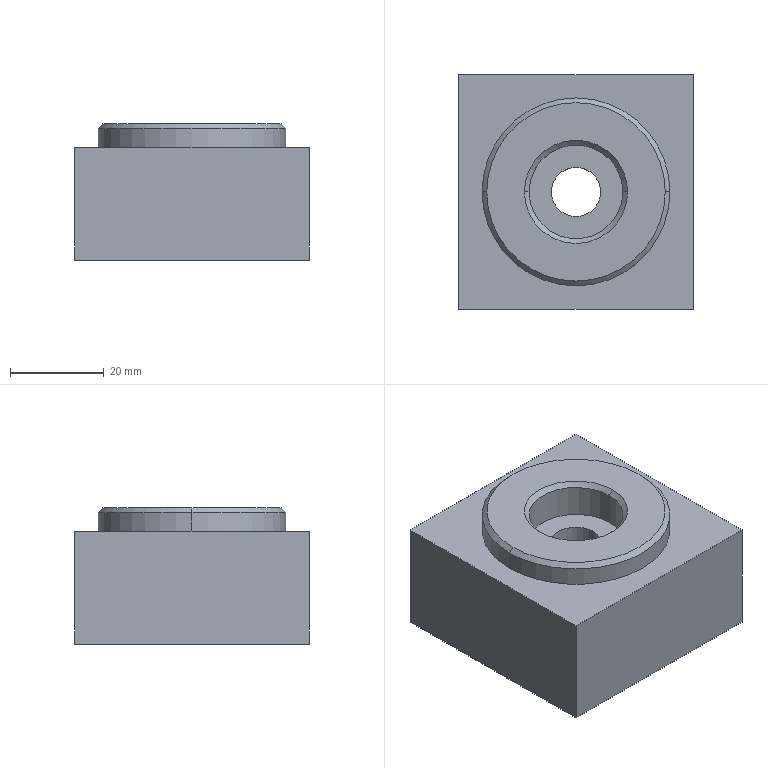Part | SolidWorks | features ICE 3, Chamfer 2, Extrusion 1 | 1 solid | 18 faces | box 50 x 50 x 29 mm | volume 61857 mm3 | plane 8 | cylinder 6 | cone 4 | commonest cylinder face diameters 10.5 x2 20 x2 40 x2
STEP:
#1=CARTESIAN_POINT('',(19.,0.,29.));
#2=VERTEX_POINT('',#1);
#3=CARTESIAN_POINT('',(-19.,0.,29.));
#4=VERTEX_POINT('',#3);
#5=CARTESIAN_POINT('',(0.,0.,29.));
#6=DIRECTION('',(0.,0.,1.));
#7=DIRECTION('',(1.,0.,0.));
#8=AXIS2_PLACEMENT_3D('',#5,#6,#7);
#9=CIRCLE('',#8,19.);
#10=EDGE_CURVE('',#2,#4,#9,.T.);
#11=ORIENTED_EDGE('',*,*,#10,.F.);
#12=CARTESIAN_POINT('',(20.,0.,28.));
#13=VERTEX_POINT('',#12);
#14=CARTESIAN_POINT('',(19.,0.,29.));
#15=DIRECTION('',(0.7071,0.,-0.7071));
#16=VECTOR('',#15,1000.);
#17=LINE('',#14,#16);
#18=EDGE_CURVE('',#2,#13,#17,.T.);
#19=ORIENTED_EDGE('',*,*,#18,.T.);
#20=CARTESIAN_POINT('',(-20.,0.,28.));
#21=VERTEX_POINT('',#20);
#22=CARTESIAN_POINT('',(0.,0.,28.));
#23=DIRECTION('',(0.,0.,-1.));
#24=DIRECTION('',(1.,0.,0.));
#25=AXIS2_PLACEMENT_3D('',#22,#23,#24);
#26=CIRCLE('',#25,20.);
#27=EDGE_CURVE('',#21,#13,#26,.T.);
#28=ORIENTED_EDGE('',*,*,#27,.F.);
#29=CARTESIAN_POINT('',(-19.,0.,29.));
#30=DIRECTION('',(-0.7071,0.,-0.7071));
#31=VECTOR('',#30,1000.);
#32=LINE('',#29,#31);
#33=EDGE_CURVE('',#4,#21,#32,.T.);
#34=ORIENTED_EDGE('',*,*,#33,.F.);
#35=EDGE_LOOP('',(#11,#19,#28,#34));
#36=FACE_OUTER_BOUND('',#35,.T.);
#37=CARTESIAN_POINT('',(0.,0.,29.));
#38=DIRECTION('',(0.,0.,-1.));
#39=DIRECTION('',(-1.,0.,0.));
#40=AXIS2_PLACEMENT_3D('',#37,#38,#39);
#41=CONICAL_SURFACE('',#40,19.,0.7854);
#42=ADVANCED_FACE('',(#36),#41,.T.);
#43=CARTESIAN_POINT('',(20.,0.,24.));
#44=VERTEX_POINT('',#43);
#45=CARTESIAN_POINT('',(-20.,0.,24.));
#46=VERTEX_POINT('',#45);
#47=CARTESIAN_POINT('',(0.,0.,24.));
#48=DIRECTION('',(0.,0.,1.));
#49=DIRECTION('',(1.,0.,0.));
#50=AXIS2_PLACEMENT_3D('',#47,#48,#49);
#51=CIRCLE('',#50,20.);
#52=EDGE_CURVE('',#44,#46,#51,.T.);
#53=ORIENTED_EDGE('',*,*,#52,.T.);
#54=CARTESIAN_POINT('',(-20.,0.,24.));
#55=DIRECTION('',(0.,0.,1.));
#56=VECTOR('',#55,1000.);
#57=LINE('',#54,#56);
#58=EDGE_CURVE('',#46,#21,#57,.T.);
#59=ORIENTED_EDGE('',*,*,#58,.T.);
#60=ORIENTED_EDGE('',*,*,#27,.T.);
#61=CARTESIAN_POINT('',(20.,0.,24.));
#62=DIRECTION('',(0.,0.,1.));
#63=VECTOR('',#62,1000.);
#64=LINE('',#61,#63);
#65=EDGE_CURVE('',#44,#13,#64,.T.);
#66=ORIENTED_EDGE('',*,*,#65,.F.);
#67=EDGE_LOOP('',(#53,#59,#60,#66));
#68=FACE_OUTER_BOUND('',#67,.T.);
#69=CARTESIAN_POINT('',(0.,0.,24.));
#70=DIRECTION('',(0.,0.,1.));
#71=DIRECTION('',(1.,0.,0.));
#72=AXIS2_PLACEMENT_3D('',#69,#70,#71);
#73=CYLINDRICAL_SURFACE('',#72,20.);
#74=ADVANCED_FACE('',(#68),#73,.T.);
#75=CARTESIAN_POINT('',(-10.,0.,28.));
#76=VERTEX_POINT('',#75);
#77=CARTESIAN_POINT('',(10.,0.,28.));
#78=VERTEX_POINT('',#77);
#79=CARTESIAN_POINT('',(0.,0.,28.));
#80=DIRECTION('',(0.,0.,1.));
#81=DIRECTION('',(1.,0.,0.));
#82=AXIS2_PLACEMENT_3D('',#79,#80,#81);
#83=CIRCLE('',#82,10.);
#84=EDGE_CURVE('',#76,#78,#83,.T.);
#85=ORIENTED_EDGE('',*,*,#84,.F.);
#86=CARTESIAN_POINT('',(-11.,0.,29.));
#87=VERTEX_POINT('',#86);
#88=CARTESIAN_POINT('',(-10.,0.,28.));
#89=DIRECTION('',(-0.7071,0.,0.7071));
#90=VECTOR('',#89,1000.);
#91=LINE('',#88,#90);
#92=EDGE_CURVE('',#76,#87,#91,.T.);
#93=ORIENTED_EDGE('',*,*,#92,.T.);
#94=CARTESIAN_POINT('',(11.,0.,29.));
#95=VERTEX_POINT('',#94);
#96=CARTESIAN_POINT('',(0.,0.,29.));
#97=DIRECTION('',(0.,0.,-1.));
#98=DIRECTION('',(1.,0.,0.));
#99=AXIS2_PLACEMENT_3D('',#96,#97,#98);
#100=CIRCLE('',#99,11.);
#101=EDGE_CURVE('',#95,#87,#100,.T.);
#102=ORIENTED_EDGE('',*,*,#101,.F.);
#103=CARTESIAN_POINT('',(10.,0.,28.));
#104=DIRECTION('',(0.7071,0.,0.7071));
#105=VECTOR('',#104,1000.);
#106=LINE('',#103,#105);
#107=EDGE_CURVE('',#78,#95,#106,.T.);
#108=ORIENTED_EDGE('',*,*,#107,.F.);
#109=EDGE_LOOP('',(#85,#93,#102,#108));
#110=FACE_OUTER_BOUND('',#109,.T.);
#111=CARTESIAN_POINT('',(0.,0.,28.));
#112=DIRECTION('',(0.,0.,1.));
#113=DIRECTION('',(1.,0.,0.));
#114=AXIS2_PLACEMENT_3D('',#111,#112,#113);
#115=CONICAL_SURFACE('',#114,10.,0.7854);
#116=ADVANCED_FACE('',(#110),#115,.F.);
#117=CARTESIAN_POINT('',(5.25,0.,21.));
#118=VERTEX_POINT('',#117);
#119=CARTESIAN_POINT('',(-5.25,0.,21.));
#120=VERTEX_POINT('',#119);
#121=CARTESIAN_POINT('',(0.,0.,21.));
#122=DIRECTION('',(0.,0.,-1.));
#123=DIRECTION('',(-1.,0.,0.));
#124=AXIS2_PLACEMENT_3D('',#121,#122,#123);
#125=CIRCLE('',#124,5.25);
#126=EDGE_CURVE('',#118,#120,#125,.T.);
#127=ORIENTED_EDGE('',*,*,#126,.F.);
#128=CARTESIAN_POINT('',(5.25,0.,0.));
#129=VERTEX_POINT('',#128);
#130=CARTESIAN_POINT('',(5.25,0.,21.));
#131=DIRECTION('',(0.,0.,-1.));
#132=VECTOR('',#131,1000.);
#133=LINE('',#130,#132);
#134=EDGE_CURVE('',#118,#129,#133,.T.);
#135=ORIENTED_EDGE('',*,*,#134,.T.);
#136=CARTESIAN_POINT('',(-5.25,0.,0.));
#137=VERTEX_POINT('',#136);
#138=CARTESIAN_POINT('',(0.,0.,0.));
#139=DIRECTION('',(0.,0.,-1.));
#140=DIRECTION('',(-1.,0.,0.));
#141=AXIS2_PLACEMENT_3D('',#138,#139,#140);
#142=CIRCLE('',#141,5.25);
#143=EDGE_CURVE('',#129,#137,#142,.T.);
#144=ORIENTED_EDGE('',*,*,#143,.T.);
#145=CARTESIAN_POINT('',(-5.25,0.,21.));
#146=DIRECTION('',(0.,0.,-1.));
#147=VECTOR('',#146,1000.);
#148=LINE('',#145,#147);
#149=EDGE_CURVE('',#120,#137,#148,.T.);
#150=ORIENTED_EDGE('',*,*,#149,.F.);
#151=EDGE_LOOP('',(#127,#135,#144,#150));
#152=FACE_OUTER_BOUND('',#151,.T.);
#153=CARTESIAN_POINT('',(0.,0.,21.));
#154=DIRECTION('',(0.,0.,-1.));
#155=DIRECTION('',(-1.,0.,0.));
#156=AXIS2_PLACEMENT_3D('',#153,#154,#155);
#157=CYLINDRICAL_SURFACE('',#156,5.25);
#158=ADVANCED_FACE('',(#152),#157,.F.);
#159=CARTESIAN_POINT('',(-10.,0.,21.));
#160=VERTEX_POINT('',#159);
#161=CARTESIAN_POINT('',(10.,0.,21.));
#162=VERTEX_POINT('',#161);
#163=CARTESIAN_POINT('',(0.,0.,21.));
#164=DIRECTION('',(0.,0.,1.));
#165=DIRECTION('',(1.,0.,0.));
#166=AXIS2_PLACEMENT_3D('',#163,#164,#165);
#167=CIRCLE('',#166,10.);
#168=EDGE_CURVE('',#160,#162,#167,.T.);
#169=ORIENTED_EDGE('',*,*,#168,.F.);
#170=CARTESIAN_POINT('',(-10.,0.,21.));
#171=DIRECTION('',(0.,0.,1.));
#172=VECTOR('',#171,1000.);
#173=LINE('',#170,#172);
#174=EDGE_CURVE('',#160,#76,#173,.T.);
#175=ORIENTED_EDGE('',*,*,#174,.T.);
#176=ORIENTED_EDGE('',*,*,#84,.T.);
#177=CARTESIAN_POINT('',(10.,0.,21.));
#178=DIRECTION('',(0.,0.,1.));
#179=VECTOR('',#178,1000.);
#180=LINE('',#177,#179);
#181=EDGE_CURVE('',#162,#78,#180,.T.);
#182=ORIENTED_EDGE('',*,*,#181,.F.);
#183=EDGE_LOOP('',(#169,#175,#176,#182));
#184=FACE_OUTER_BOUND('',#183,.T.);
#185=CARTESIAN_POINT('',(0.,0.,21.));
#186=DIRECTION('',(0.,0.,1.));
#187=DIRECTION('',(1.,0.,0.));
#188=AXIS2_PLACEMENT_3D('',#185,#186,#187);
#189=CYLINDRICAL_SURFACE('',#188,10.);
#190=ADVANCED_FACE('',(#184),#189,.F.);
#191=CARTESIAN_POINT('',(25.,-25.,24.));
#192=VERTEX_POINT('',#191);
#193=CARTESIAN_POINT('',(25.,25.,24.));
#194=VERTEX_POINT('',#193);
#195=CARTESIAN_POINT('',(25.,25.,24.));
#196=DIRECTION('',(0.,1.,0.));
#197=VECTOR('',#196,1000.);
#198=LINE('',#195,#197);
#199=EDGE_CURVE('',#192,#194,#198,.T.);
#200=ORIENTED_EDGE('',*,*,#199,.F.);
#201=CARTESIAN_POINT('',(25.,-25.,0.));
#202=VERTEX_POINT('',#201);
#203=CARTESIAN_POINT('',(25.,-25.,29.));
#204=DIRECTION('',(0.,0.,-1.));
#205=VECTOR('',#204,1000.);
#206=LINE('',#203,#205);
#207=EDGE_CURVE('',#192,#202,#206,.T.);
#208=ORIENTED_EDGE('',*,*,#207,.T.);
#209=CARTESIAN_POINT('',(25.,25.,0.));
#210=VERTEX_POINT('',#209);
#211=CARTESIAN_POINT('',(25.,25.,0.));
#212=DIRECTION('',(0.,1.,0.));
#213=VECTOR('',#212,1000.);
#214=LINE('',#211,#213);
#215=EDGE_CURVE('',#202,#210,#214,.T.);
#216=ORIENTED_EDGE('',*,*,#215,.T.);
#217=CARTESIAN_POINT('',(25.,25.,29.));
#218=DIRECTION('',(0.,0.,-1.));
#219=VECTOR('',#218,1000.);
#220=LINE('',#217,#219);
#221=EDGE_CURVE('',#194,#210,#220,.T.);
#222=ORIENTED_EDGE('',*,*,#221,.F.);
#223=EDGE_LOOP('',(#200,#208,#216,#222));
#224=FACE_OUTER_BOUND('',#223,.T.);
#225=CARTESIAN_POINT('',(25.,25.,29.));
#226=DIRECTION('',(-1.,0.,0.));
#227=DIRECTION('',(0.,-1.,0.));
#228=AXIS2_PLACEMENT_3D('',#225,#226,#227);
#229=PLANE('',#228);
#230=ADVANCED_FACE('',(#224),#229,.F.);
#231=CARTESIAN_POINT('',(-25.,25.,24.));
#232=VERTEX_POINT('',#231);
#233=CARTESIAN_POINT('',(-25.,25.,24.));
#234=DIRECTION('',(-1.,0.,0.));
#235=VECTOR('',#234,1000.);
#236=LINE('',#233,#235);
#237=EDGE_CURVE('',#194,#232,#236,.T.);
#238=ORIENTED_EDGE('',*,*,#237,.F.);
#239=ORIENTED_EDGE('',*,*,#221,.T.);
#240=CARTESIAN_POINT('',(-25.,25.,0.));
#241=VERTEX_POINT('',#240);
#242=CARTESIAN_POINT('',(-25.,25.,0.));
#243=DIRECTION('',(-1.,0.,0.));
#244=VECTOR('',#243,1000.);
#245=LINE('',#242,#244);
#246=EDGE_CURVE('',#210,#241,#245,.T.);
#247=ORIENTED_EDGE('',*,*,#246,.T.);
#248=CARTESIAN_POINT('',(-25.,25.,29.));
#249=DIRECTION('',(0.,0.,-1.));
#250=VECTOR('',#249,1000.);
#251=LINE('',#248,#250);
#252=EDGE_CURVE('',#232,#241,#251,.T.);
#253=ORIENTED_EDGE('',*,*,#252,.F.);
#254=EDGE_LOOP('',(#238,#239,#247,#253));
#255=FACE_OUTER_BOUND('',#254,.T.);
#256=CARTESIAN_POINT('',(-25.,25.,29.));
#257=DIRECTION('',(0.,-1.,0.));
#258=DIRECTION('',(0.,0.,-1.));
#259=AXIS2_PLACEMENT_3D('',#256,#257,#258);
#260=PLANE('',#259);
#261=ADVANCED_FACE('',(#255),#260,.F.);
#262=CARTESIAN_POINT('',(-25.,-25.,24.));
#263=VERTEX_POINT('',#262);
#264=CARTESIAN_POINT('',(-25.,25.,24.));
#265=DIRECTION('',(0.,-1.,0.));
#266=VECTOR('',#265,1000.);
#267=LINE('',#264,#266);
#268=EDGE_CURVE('',#232,#263,#267,.T.);
#269=ORIENTED_EDGE('',*,*,#268,.F.);
#270=ORIENTED_EDGE('',*,*,#252,.T.);
#271=CARTESIAN_POINT('',(-25.,-25.,0.));
#272=VERTEX_POINT('',#271);
#273=CARTESIAN_POINT('',(-25.,25.,0.));
#274=DIRECTION('',(0.,-1.,0.));
#275=VECTOR('',#274,1000.);
#276=LINE('',#273,#275);
#277=EDGE_CURVE('',#241,#272,#276,.T.);
#278=ORIENTED_EDGE('',*,*,#277,.T.);
#279=CARTESIAN_POINT('',(-25.,-25.,29.));
#280=DIRECTION('',(0.,0.,-1.));
#281=VECTOR('',#280,1000.);
#282=LINE('',#279,#281);
#283=EDGE_CURVE('',#263,#272,#282,.T.);
#284=ORIENTED_EDGE('',*,*,#283,.F.);
#285=EDGE_LOOP('',(#269,#270,#278,#284));
#286=FACE_OUTER_BOUND('',#285,.T.);
#287=CARTESIAN_POINT('',(-25.,25.,29.));
#288=DIRECTION('',(1.,0.,0.));
#289=DIRECTION('',(0.,1.,0.));
#290=AXIS2_PLACEMENT_3D('',#287,#288,#289);
#291=PLANE('',#290);
#292=ADVANCED_FACE('',(#286),#291,.F.);
#293=CARTESIAN_POINT('',(-25.,-25.,24.));
#294=DIRECTION('',(1.,0.,0.));
#295=VECTOR('',#294,1000.);
#296=LINE('',#293,#295);
#297=EDGE_CURVE('',#263,#192,#296,.T.);
#298=ORIENTED_EDGE('',*,*,#297,.F.);
#299=ORIENTED_EDGE('',*,*,#283,.T.);
#300=CARTESIAN_POINT('',(-25.,-25.,0.));
#301=DIRECTION('',(1.,0.,0.));
#302=VECTOR('',#301,1000.);
#303=LINE('',#300,#302);
#304=EDGE_CURVE('',#272,#202,#303,.T.);
#305=ORIENTED_EDGE('',*,*,#304,.T.);
#306=ORIENTED_EDGE('',*,*,#207,.F.);
#307=EDGE_LOOP('',(#298,#299,#305,#306));
#308=FACE_OUTER_BOUND('',#307,.T.);
#309=CARTESIAN_POINT('',(-25.,-25.,29.));
#310=DIRECTION('',(0.,1.,0.));
#311=DIRECTION('',(0.,0.,1.));
#312=AXIS2_PLACEMENT_3D('',#309,#310,#311);
#313=PLANE('',#312);
#314=ADVANCED_FACE('',(#308),#313,.F.);
#315=CARTESIAN_POINT('',(0.,0.,29.));
#316=DIRECTION('',(0.,0.,1.));
#317=DIRECTION('',(1.,0.,0.));
#318=AXIS2_PLACEMENT_3D('',#315,#316,#317);
#319=CIRCLE('',#318,19.);
#320=EDGE_CURVE('',#4,#2,#319,.T.);
#321=ORIENTED_EDGE('',*,*,#320,.T.);
#322=ORIENTED_EDGE('',*,*,#10,.T.);
#323=EDGE_LOOP('',(#321,#322));
#324=FACE_OUTER_BOUND('',#323,.T.);
#325=ORIENTED_EDGE('',*,*,#101,.T.);
#326=CARTESIAN_POINT('',(0.,0.,29.));
#327=DIRECTION('',(0.,0.,-1.));
#328=DIRECTION('',(1.,0.,0.));
#329=AXIS2_PLACEMENT_3D('',#326,#327,#328);
#330=CIRCLE('',#329,11.);
#331=EDGE_CURVE('',#87,#95,#330,.T.);
#332=ORIENTED_EDGE('',*,*,#331,.T.);
#333=EDGE_LOOP('',(#325,#332));
#334=FACE_BOUND('',#333,.T.);
#335=CARTESIAN_POINT('',(0.,0.,29.));
#336=DIRECTION('',(0.,0.,1.));
#337=DIRECTION('',(1.,0.,0.));
#338=AXIS2_PLACEMENT_3D('',#335,#336,#337);
#339=PLANE('',#338);
#340=ADVANCED_FACE('',(#324,#334),#339,.T.);
#341=CARTESIAN_POINT('',(0.,0.,0.));
#342=DIRECTION('',(0.,0.,-1.));
#343=DIRECTION('',(-1.,0.,0.));
#344=AXIS2_PLACEMENT_3D('',#341,#342,#343);
#345=CIRCLE('',#344,5.25);
#346=EDGE_CURVE('',#137,#129,#345,.T.);
#347=ORIENTED_EDGE('',*,*,#346,.F.);
#348=ORIENTED_EDGE('',*,*,#143,.F.);
#349=EDGE_LOOP('',(#347,#348));
#350=FACE_BOUND('',#349,.T.);
#351=ORIENTED_EDGE('',*,*,#215,.F.);
#352=ORIENTED_EDGE('',*,*,#304,.F.);
#353=ORIENTED_EDGE('',*,*,#277,.F.);
#354=ORIENTED_EDGE('',*,*,#246,.F.);
#355=EDGE_LOOP('',(#351,#352,#353,#354));
#356=FACE_OUTER_BOUND('',#355,.T.);
#357=CARTESIAN_POINT('',(0.,0.,0.));
#358=DIRECTION('',(0.,0.,1.));
#359=DIRECTION('',(1.,0.,0.));
#360=AXIS2_PLACEMENT_3D('',#357,#358,#359);
#361=PLANE('',#360);
#362=ADVANCED_FACE('',(#350,#356),#361,.F.);
#363=ORIENTED_EDGE('',*,*,#174,.F.);
#364=CARTESIAN_POINT('',(0.,0.,21.));
#365=DIRECTION('',(0.,0.,1.));
#366=DIRECTION('',(1.,0.,0.));
#367=AXIS2_PLACEMENT_3D('',#364,#365,#366);
#368=CIRCLE('',#367,10.);
#369=EDGE_CURVE('',#162,#160,#368,.T.);
#370=ORIENTED_EDGE('',*,*,#369,.F.);
#371=ORIENTED_EDGE('',*,*,#181,.T.);
#372=CARTESIAN_POINT('',(0.,0.,28.));
#373=DIRECTION('',(0.,0.,1.));
#374=DIRECTION('',(1.,0.,0.));
#375=AXIS2_PLACEMENT_3D('',#372,#373,#374);
#376=CIRCLE('',#375,10.);
#377=EDGE_CURVE('',#78,#76,#376,.T.);
#378=ORIENTED_EDGE('',*,*,#377,.T.);
#379=EDGE_LOOP('',(#363,#370,#371,#378));
#380=FACE_OUTER_BOUND('',#379,.T.);
#381=CARTESIAN_POINT('',(0.,0.,21.));
#382=DIRECTION('',(0.,0.,1.));
#383=DIRECTION('',(1.,0.,0.));
#384=AXIS2_PLACEMENT_3D('',#381,#382,#383);
#385=CYLINDRICAL_SURFACE('',#384,10.);
#386=ADVANCED_FACE('',(#380),#385,.F.);
#387=CARTESIAN_POINT('',(0.,0.,21.));
#388=DIRECTION('',(0.,0.,-1.));
#389=DIRECTION('',(-1.,0.,0.));
#390=AXIS2_PLACEMENT_3D('',#387,#388,#389);
#391=CIRCLE('',#390,5.25);
#392=EDGE_CURVE('',#120,#118,#391,.T.);
#393=ORIENTED_EDGE('',*,*,#392,.T.);
#394=ORIENTED_EDGE('',*,*,#126,.T.);
#395=EDGE_LOOP('',(#393,#394));
#396=FACE_BOUND('',#395,.T.);
#397=ORIENTED_EDGE('',*,*,#369,.T.);
#398=ORIENTED_EDGE('',*,*,#168,.T.);
#399=EDGE_LOOP('',(#397,#398));
#400=FACE_OUTER_BOUND('',#399,.T.);
#401=CARTESIAN_POINT('',(0.,0.,21.));
#402=DIRECTION('',(0.,0.,1.));
#403=DIRECTION('',(1.,0.,0.));
#404=AXIS2_PLACEMENT_3D('',#401,#402,#403);
#405=PLANE('',#404);
#406=ADVANCED_FACE('',(#396,#400),#405,.T.);
#407=ORIENTED_EDGE('',*,*,#134,.F.);
#408=ORIENTED_EDGE('',*,*,#392,.F.);
#409=ORIENTED_EDGE('',*,*,#149,.T.);
#410=ORIENTED_EDGE('',*,*,#346,.T.);
#411=EDGE_LOOP('',(#407,#408,#409,#410));
#412=FACE_OUTER_BOUND('',#411,.T.);
#413=CARTESIAN_POINT('',(0.,0.,21.));
#414=DIRECTION('',(0.,0.,-1.));
#415=DIRECTION('',(-1.,0.,0.));
#416=AXIS2_PLACEMENT_3D('',#413,#414,#415);
#417=CYLINDRICAL_SURFACE('',#416,5.25);
#418=ADVANCED_FACE('',(#412),#417,.F.);
#419=ORIENTED_EDGE('',*,*,#92,.F.);
#420=ORIENTED_EDGE('',*,*,#377,.F.);
#421=ORIENTED_EDGE('',*,*,#107,.T.);
#422=ORIENTED_EDGE('',*,*,#331,.F.);
#423=EDGE_LOOP('',(#419,#420,#421,#422));
#424=FACE_OUTER_BOUND('',#423,.T.);
#425=CARTESIAN_POINT('',(0.,0.,28.));
#426=DIRECTION('',(0.,0.,1.));
#427=DIRECTION('',(1.,0.,0.));
#428=AXIS2_PLACEMENT_3D('',#425,#426,#427);
#429=CONICAL_SURFACE('',#428,10.,0.7854);
#430=ADVANCED_FACE('',(#424),#429,.F.);
#431=ORIENTED_EDGE('',*,*,#52,.F.);
#432=CARTESIAN_POINT('',(0.,0.,24.));
#433=DIRECTION('',(0.,0.,1.));
#434=DIRECTION('',(1.,0.,0.));
#435=AXIS2_PLACEMENT_3D('',#432,#433,#434);
#436=CIRCLE('',#435,20.);
#437=EDGE_CURVE('',#46,#44,#436,.T.);
#438=ORIENTED_EDGE('',*,*,#437,.F.);
#439=EDGE_LOOP('',(#431,#438));
#440=FACE_BOUND('',#439,.T.);
#441=ORIENTED_EDGE('',*,*,#199,.T.);
#442=ORIENTED_EDGE('',*,*,#237,.T.);
#443=ORIENTED_EDGE('',*,*,#268,.T.);
#444=ORIENTED_EDGE('',*,*,#297,.T.);
#445=EDGE_LOOP('',(#441,#442,#443,#444));
#446=FACE_OUTER_BOUND('',#445,.T.);
#447=CARTESIAN_POINT('',(0.,0.,24.));
#448=DIRECTION('',(0.,0.,1.));
#449=DIRECTION('',(1.,0.,0.));
#450=AXIS2_PLACEMENT_3D('',#447,#448,#449);
#451=PLANE('',#450);
#452=ADVANCED_FACE('',(#440,#446),#451,.T.);
#453=ORIENTED_EDGE('',*,*,#58,.F.);
#454=ORIENTED_EDGE('',*,*,#437,.T.);
#455=ORIENTED_EDGE('',*,*,#65,.T.);
#456=CARTESIAN_POINT('',(0.,0.,28.));
#457=DIRECTION('',(0.,0.,-1.));
#458=DIRECTION('',(1.,0.,0.));
#459=AXIS2_PLACEMENT_3D('',#456,#457,#458);
#460=CIRCLE('',#459,20.);
#461=EDGE_CURVE('',#13,#21,#460,.T.);
#462=ORIENTED_EDGE('',*,*,#461,.T.);
#463=EDGE_LOOP('',(#453,#454,#455,#462));
#464=FACE_OUTER_BOUND('',#463,.T.);
#465=CARTESIAN_POINT('',(0.,0.,24.));
#466=DIRECTION('',(0.,0.,1.));
#467=DIRECTION('',(1.,0.,0.));
#468=AXIS2_PLACEMENT_3D('',#465,#466,#467);
#469=CYLINDRICAL_SURFACE('',#468,20.);
#470=ADVANCED_FACE('',(#464),#469,.T.);
#471=ORIENTED_EDGE('',*,*,#18,.F.);
#472=ORIENTED_EDGE('',*,*,#320,.F.);
#473=ORIENTED_EDGE('',*,*,#33,.T.);
#474=ORIENTED_EDGE('',*,*,#461,.F.);
#475=EDGE_LOOP('',(#471,#472,#473,#474));
#476=FACE_OUTER_BOUND('',#475,.T.);
#477=CARTESIAN_POINT('',(0.,0.,29.));
#478=DIRECTION('',(0.,0.,-1.));
#479=DIRECTION('',(-1.,0.,0.));
#480=AXIS2_PLACEMENT_3D('',#477,#478,#479);
#481=CONICAL_SURFACE('',#480,19.,0.7854);
#482=ADVANCED_FACE('',(#476),#481,.T.);
#483=CLOSED_SHELL('',(#42,#74,#116,#158,#190,#230,#261,#292,#314,#340,#362,#386,#406,#418,#430,#452,#470,#482));
#484=MANIFOLD_SOLID_BREP('',#483);
#485=CARTESIAN_POINT('',(0.,0.,0.));
#486=DIRECTION('',(0.,0.,1.));
#487=DIRECTION('',(1.,0.,0.));
#488=AXIS2_PLACEMENT_3D('',#485,#486,#487);
#489=(LENGTH_UNIT()NAMED_UNIT(*)SI_UNIT(.MILLI.,.METRE.));
#490=UNCERTAINTY_MEASURE_WITH_UNIT(LENGTH_MEASURE(0.00001),#489,'','');
#491=(NAMED_UNIT(*)PLANE_ANGLE_UNIT()SI_UNIT($,.RADIAN.));
#492=(NAMED_UNIT(*)SI_UNIT($,.STERADIAN.)SOLID_ANGLE_UNIT());
#493=(GEOMETRIC_REPRESENTATION_CONTEXT(3)GLOBAL_UNCERTAINTY_ASSIGNED_CONTEXT((#490))GLOBAL_UNIT_ASSIGNED_CONTEXT((#489,#491,#492))REPRESENTATION_CONTEXT('',''));
#494=ADVANCED_BREP_SHAPE_REPRESENTATION('',(#484,#488),#493);